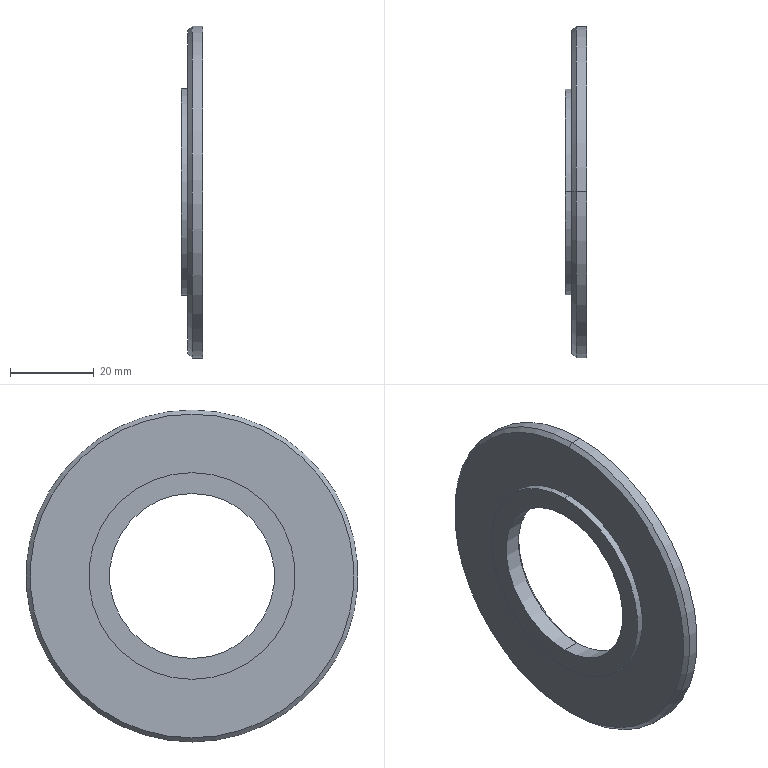Part | SolidWorks | features Chamfer 2, Revolution 1 | 1 solid | 13 faces | box 5.21 x 79.5 x 79.5 mm | volume 14367 mm3 | cylinder 6 | cone 4 | plane 3 | commonest cylinder face diameters 39.5 x2 49.5 x2 79.5 x2
STEP:
#1=CARTESIAN_POINT('',(10.713,-22.417,19.75));
#2=VERTEX_POINT('',#1);
#3=CARTESIAN_POINT('',(10.713,-22.417,-19.75));
#4=VERTEX_POINT('',#3);
#5=CARTESIAN_POINT('',(10.713,-22.417,0.));
#6=DIRECTION('',(1.,0.,0.));
#7=DIRECTION('',(0.,0.,1.));
#8=AXIS2_PLACEMENT_3D('',#5,#6,#7);
#9=CIRCLE('',#8,19.75);
#10=EDGE_CURVE('',#2,#4,#9,.T.);
#11=ORIENTED_EDGE('',*,*,#10,.F.);
#12=CARTESIAN_POINT('',(11.713,-22.417,20.75));
#13=VERTEX_POINT('',#12);
#14=CARTESIAN_POINT('',(11.713,-22.417,20.75));
#15=DIRECTION('',(0.7071,0.,0.7071));
#16=VECTOR('',#15,1000.);
#17=LINE('',#14,#16);
#18=EDGE_CURVE('',#2,#13,#17,.T.);
#19=ORIENTED_EDGE('',*,*,#18,.T.);
#20=CARTESIAN_POINT('',(11.713,-22.417,-20.75));
#21=VERTEX_POINT('',#20);
#22=CARTESIAN_POINT('',(11.713,-22.417,0.));
#23=DIRECTION('',(-1.,0.,0.));
#24=DIRECTION('',(0.,0.,1.));
#25=AXIS2_PLACEMENT_3D('',#22,#23,#24);
#26=CIRCLE('',#25,20.75);
#27=EDGE_CURVE('',#21,#13,#26,.T.);
#28=ORIENTED_EDGE('',*,*,#27,.F.);
#29=CARTESIAN_POINT('',(11.713,-22.417,-20.75));
#30=DIRECTION('',(0.7071,0.,-0.7071));
#31=VECTOR('',#30,1000.);
#32=LINE('',#29,#31);
#33=EDGE_CURVE('',#4,#21,#32,.T.);
#34=ORIENTED_EDGE('',*,*,#33,.F.);
#35=EDGE_LOOP('',(#11,#19,#28,#34));
#36=FACE_OUTER_BOUND('',#35,.T.);
#37=CARTESIAN_POINT('',(11.713,-22.417,0.));
#38=DIRECTION('',(1.,0.,0.));
#39=DIRECTION('',(0.,0.,-1.));
#40=AXIS2_PLACEMENT_3D('',#37,#38,#39);
#41=CONICAL_SURFACE('',#40,20.75,0.7854);
#42=ADVANCED_FACE('',(#36),#41,.F.);
#43=CARTESIAN_POINT('',(8.123,-22.417,38.75));
#44=VERTEX_POINT('',#43);
#45=CARTESIAN_POINT('',(8.123,-22.417,-38.75));
#46=VERTEX_POINT('',#45);
#47=CARTESIAN_POINT('',(8.123,-22.417,0.));
#48=DIRECTION('',(-1.,0.,0.));
#49=DIRECTION('',(0.,0.,-1.));
#50=AXIS2_PLACEMENT_3D('',#47,#48,#49);
#51=CIRCLE('',#50,38.75);
#52=EDGE_CURVE('',#44,#46,#51,.T.);
#53=ORIENTED_EDGE('',*,*,#52,.F.);
#54=CARTESIAN_POINT('',(9.123,-22.417,39.75));
#55=VERTEX_POINT('',#54);
#56=CARTESIAN_POINT('',(8.123,-22.417,38.75));
#57=DIRECTION('',(0.7071,0.,0.7071));
#58=VECTOR('',#57,1000.);
#59=LINE('',#56,#58);
#60=EDGE_CURVE('',#44,#55,#59,.T.);
#61=ORIENTED_EDGE('',*,*,#60,.T.);
#62=CARTESIAN_POINT('',(9.123,-22.417,-39.75));
#63=VERTEX_POINT('',#62);
#64=CARTESIAN_POINT('',(9.123,-22.417,0.));
#65=DIRECTION('',(1.,0.,0.));
#66=DIRECTION('',(0.,0.,-1.));
#67=AXIS2_PLACEMENT_3D('',#64,#65,#66);
#68=CIRCLE('',#67,39.75);
#69=EDGE_CURVE('',#63,#55,#68,.T.);
#70=ORIENTED_EDGE('',*,*,#69,.F.);
#71=CARTESIAN_POINT('',(8.123,-22.417,-38.75));
#72=DIRECTION('',(0.7071,0.,-0.7071));
#73=VECTOR('',#72,1000.);
#74=LINE('',#71,#73);
#75=EDGE_CURVE('',#46,#63,#74,.T.);
#76=ORIENTED_EDGE('',*,*,#75,.F.);
#77=EDGE_LOOP('',(#53,#61,#70,#76));
#78=FACE_OUTER_BOUND('',#77,.T.);
#79=CARTESIAN_POINT('',(8.123,-22.417,0.));
#80=DIRECTION('',(1.,0.,0.));
#81=DIRECTION('',(0.,0.,-1.));
#82=AXIS2_PLACEMENT_3D('',#79,#80,#81);
#83=CONICAL_SURFACE('',#82,38.75,0.7854);
#84=ADVANCED_FACE('',(#78),#83,.T.);
#85=CARTESIAN_POINT('',(8.123,-22.417,24.75));
#86=VERTEX_POINT('',#85);
#87=CARTESIAN_POINT('',(8.123,-22.417,-24.75));
#88=VERTEX_POINT('',#87);
#89=CARTESIAN_POINT('',(8.123,-22.417,0.));
#90=DIRECTION('',(-1.,0.,0.));
#91=DIRECTION('',(0.,0.,1.));
#92=AXIS2_PLACEMENT_3D('',#89,#90,#91);
#93=CIRCLE('',#92,24.75);
#94=EDGE_CURVE('',#86,#88,#93,.T.);
#95=ORIENTED_EDGE('',*,*,#94,.T.);
#96=CARTESIAN_POINT('',(6.503,-22.417,-24.75));
#97=VERTEX_POINT('',#96);
#98=CARTESIAN_POINT('',(4.025,-22.417,-24.75));
#99=DIRECTION('',(-1.,0.,0.));
#100=VECTOR('',#99,1000.);
#101=LINE('',#98,#100);
#102=EDGE_CURVE('',#88,#97,#101,.T.);
#103=ORIENTED_EDGE('',*,*,#102,.T.);
#104=CARTESIAN_POINT('',(6.503,-22.417,24.75));
#105=VERTEX_POINT('',#104);
#106=CARTESIAN_POINT('',(6.503,-22.417,0.));
#107=DIRECTION('',(-1.,0.,0.));
#108=DIRECTION('',(0.,0.,1.));
#109=AXIS2_PLACEMENT_3D('',#106,#107,#108);
#110=CIRCLE('',#109,24.75);
#111=EDGE_CURVE('',#105,#97,#110,.T.);
#112=ORIENTED_EDGE('',*,*,#111,.F.);
#113=CARTESIAN_POINT('',(4.025,-22.417,24.75));
#114=DIRECTION('',(-1.,0.,0.));
#115=VECTOR('',#114,1000.);
#116=LINE('',#113,#115);
#117=EDGE_CURVE('',#86,#105,#116,.T.);
#118=ORIENTED_EDGE('',*,*,#117,.F.);
#119=EDGE_LOOP('',(#95,#103,#112,#118));
#120=FACE_OUTER_BOUND('',#119,.T.);
#121=CARTESIAN_POINT('',(4.025,-22.417,0.));
#122=DIRECTION('',(-1.,0.,0.));
#123=DIRECTION('',(0.,0.,1.));
#124=AXIS2_PLACEMENT_3D('',#121,#122,#123);
#125=CYLINDRICAL_SURFACE('',#124,24.75);
#126=ADVANCED_FACE('',(#120),#125,.T.);
#127=ORIENTED_EDGE('',*,*,#10,.T.);
#128=CARTESIAN_POINT('',(6.503,-22.417,-19.75));
#129=VERTEX_POINT('',#128);
#130=CARTESIAN_POINT('',(4.025,-22.417,-19.75));
#131=DIRECTION('',(-1.,0.,0.));
#132=VECTOR('',#131,1000.);
#133=LINE('',#130,#132);
#134=EDGE_CURVE('',#4,#129,#133,.T.);
#135=ORIENTED_EDGE('',*,*,#134,.T.);
#136=CARTESIAN_POINT('',(6.503,-22.417,19.75));
#137=VERTEX_POINT('',#136);
#138=CARTESIAN_POINT('',(6.503,-22.417,0.));
#139=DIRECTION('',(-1.,0.,0.));
#140=DIRECTION('',(0.,0.,1.));
#141=AXIS2_PLACEMENT_3D('',#138,#139,#140);
#142=CIRCLE('',#141,19.75);
#143=EDGE_CURVE('',#129,#137,#142,.T.);
#144=ORIENTED_EDGE('',*,*,#143,.T.);
#145=CARTESIAN_POINT('',(4.025,-22.417,19.75));
#146=DIRECTION('',(-1.,0.,0.));
#147=VECTOR('',#146,1000.);
#148=LINE('',#145,#147);
#149=EDGE_CURVE('',#2,#137,#148,.T.);
#150=ORIENTED_EDGE('',*,*,#149,.F.);
#151=EDGE_LOOP('',(#127,#135,#144,#150));
#152=FACE_OUTER_BOUND('',#151,.T.);
#153=CARTESIAN_POINT('',(4.025,-22.417,0.));
#154=DIRECTION('',(-1.,0.,0.));
#155=DIRECTION('',(0.,0.,1.));
#156=AXIS2_PLACEMENT_3D('',#153,#154,#155);
#157=CYLINDRICAL_SURFACE('',#156,19.75);
#158=ADVANCED_FACE('',(#152),#157,.F.);
#159=CARTESIAN_POINT('',(11.713,-22.417,39.75));
#160=VERTEX_POINT('',#159);
#161=CARTESIAN_POINT('',(11.713,-22.417,-39.75));
#162=VERTEX_POINT('',#161);
#163=CARTESIAN_POINT('',(11.713,-22.417,0.));
#164=DIRECTION('',(-1.,0.,0.));
#165=DIRECTION('',(0.,0.,1.));
#166=AXIS2_PLACEMENT_3D('',#163,#164,#165);
#167=CIRCLE('',#166,39.75);
#168=EDGE_CURVE('',#160,#162,#167,.T.);
#169=ORIENTED_EDGE('',*,*,#168,.T.);
#170=CARTESIAN_POINT('',(4.025,-22.417,-39.75));
#171=DIRECTION('',(-1.,0.,0.));
#172=VECTOR('',#171,1000.);
#173=LINE('',#170,#172);
#174=EDGE_CURVE('',#162,#63,#173,.T.);
#175=ORIENTED_EDGE('',*,*,#174,.T.);
#176=ORIENTED_EDGE('',*,*,#69,.T.);
#177=CARTESIAN_POINT('',(4.025,-22.417,39.75));
#178=DIRECTION('',(-1.,0.,0.));
#179=VECTOR('',#178,1000.);
#180=LINE('',#177,#179);
#181=EDGE_CURVE('',#160,#55,#180,.T.);
#182=ORIENTED_EDGE('',*,*,#181,.F.);
#183=EDGE_LOOP('',(#169,#175,#176,#182));
#184=FACE_OUTER_BOUND('',#183,.T.);
#185=CARTESIAN_POINT('',(4.025,-22.417,0.));
#186=DIRECTION('',(-1.,0.,0.));
#187=DIRECTION('',(0.,0.,1.));
#188=AXIS2_PLACEMENT_3D('',#185,#186,#187);
#189=CYLINDRICAL_SURFACE('',#188,39.75);
#190=ADVANCED_FACE('',(#184),#189,.T.);
#191=CARTESIAN_POINT('',(8.123,-22.417,0.));
#192=DIRECTION('',(-1.,0.,0.));
#193=DIRECTION('',(0.,0.,-1.));
#194=AXIS2_PLACEMENT_3D('',#191,#192,#193);
#195=CIRCLE('',#194,38.75);
#196=EDGE_CURVE('',#46,#44,#195,.T.);
#197=ORIENTED_EDGE('',*,*,#196,.T.);
#198=ORIENTED_EDGE('',*,*,#52,.T.);
#199=EDGE_LOOP('',(#197,#198));
#200=FACE_OUTER_BOUND('',#199,.T.);
#201=ORIENTED_EDGE('',*,*,#94,.F.);
#202=CARTESIAN_POINT('',(8.123,-22.417,0.));
#203=DIRECTION('',(-1.,0.,0.));
#204=DIRECTION('',(0.,0.,1.));
#205=AXIS2_PLACEMENT_3D('',#202,#203,#204);
#206=CIRCLE('',#205,24.75);
#207=EDGE_CURVE('',#88,#86,#206,.T.);
#208=ORIENTED_EDGE('',*,*,#207,.F.);
#209=EDGE_LOOP('',(#201,#208));
#210=FACE_BOUND('',#209,.T.);
#211=CARTESIAN_POINT('',(8.123,2.333,0.));
#212=DIRECTION('',(1.,0.,0.));
#213=DIRECTION('',(0.,0.,-1.));
#214=AXIS2_PLACEMENT_3D('',#211,#212,#213);
#215=PLANE('',#214);
#216=ADVANCED_FACE('',(#200,#210),#215,.F.);
#217=ORIENTED_EDGE('',*,*,#174,.F.);
#218=CARTESIAN_POINT('',(11.713,-22.417,0.));
#219=DIRECTION('',(-1.,0.,0.));
#220=DIRECTION('',(0.,0.,1.));
#221=AXIS2_PLACEMENT_3D('',#218,#219,#220);
#222=CIRCLE('',#221,39.75);
#223=EDGE_CURVE('',#162,#160,#222,.T.);
#224=ORIENTED_EDGE('',*,*,#223,.T.);
#225=ORIENTED_EDGE('',*,*,#181,.T.);
#226=CARTESIAN_POINT('',(9.123,-22.417,0.));
#227=DIRECTION('',(1.,0.,0.));
#228=DIRECTION('',(0.,0.,-1.));
#229=AXIS2_PLACEMENT_3D('',#226,#227,#228);
#230=CIRCLE('',#229,39.75);
#231=EDGE_CURVE('',#55,#63,#230,.T.);
#232=ORIENTED_EDGE('',*,*,#231,.T.);
#233=EDGE_LOOP('',(#217,#224,#225,#232));
#234=FACE_OUTER_BOUND('',#233,.T.);
#235=CARTESIAN_POINT('',(4.025,-22.417,0.));
#236=DIRECTION('',(-1.,0.,0.));
#237=DIRECTION('',(0.,0.,1.));
#238=AXIS2_PLACEMENT_3D('',#235,#236,#237);
#239=CYLINDRICAL_SURFACE('',#238,39.75);
#240=ADVANCED_FACE('',(#234),#239,.T.);
#241=ORIENTED_EDGE('',*,*,#27,.T.);
#242=CARTESIAN_POINT('',(11.713,-22.417,0.));
#243=DIRECTION('',(-1.,0.,0.));
#244=DIRECTION('',(0.,0.,1.));
#245=AXIS2_PLACEMENT_3D('',#242,#243,#244);
#246=CIRCLE('',#245,20.75);
#247=EDGE_CURVE('',#13,#21,#246,.T.);
#248=ORIENTED_EDGE('',*,*,#247,.T.);
#249=EDGE_LOOP('',(#241,#248));
#250=FACE_BOUND('',#249,.T.);
#251=ORIENTED_EDGE('',*,*,#168,.F.);
#252=ORIENTED_EDGE('',*,*,#223,.F.);
#253=EDGE_LOOP('',(#251,#252));
#254=FACE_OUTER_BOUND('',#253,.T.);
#255=CARTESIAN_POINT('',(11.713,17.333,0.));
#256=DIRECTION('',(-1.,0.,0.));
#257=DIRECTION('',(0.,0.,1.));
#258=AXIS2_PLACEMENT_3D('',#255,#256,#257);
#259=PLANE('',#258);
#260=ADVANCED_FACE('',(#250,#254),#259,.F.);
#261=ORIENTED_EDGE('',*,*,#134,.F.);
#262=CARTESIAN_POINT('',(10.713,-22.417,0.));
#263=DIRECTION('',(1.,0.,0.));
#264=DIRECTION('',(0.,0.,1.));
#265=AXIS2_PLACEMENT_3D('',#262,#263,#264);
#266=CIRCLE('',#265,19.75);
#267=EDGE_CURVE('',#4,#2,#266,.T.);
#268=ORIENTED_EDGE('',*,*,#267,.T.);
#269=ORIENTED_EDGE('',*,*,#149,.T.);
#270=CARTESIAN_POINT('',(6.503,-22.417,0.));
#271=DIRECTION('',(-1.,0.,0.));
#272=DIRECTION('',(0.,0.,1.));
#273=AXIS2_PLACEMENT_3D('',#270,#271,#272);
#274=CIRCLE('',#273,19.75);
#275=EDGE_CURVE('',#137,#129,#274,.T.);
#276=ORIENTED_EDGE('',*,*,#275,.T.);
#277=EDGE_LOOP('',(#261,#268,#269,#276));
#278=FACE_OUTER_BOUND('',#277,.T.);
#279=CARTESIAN_POINT('',(4.025,-22.417,0.));
#280=DIRECTION('',(-1.,0.,0.));
#281=DIRECTION('',(0.,0.,1.));
#282=AXIS2_PLACEMENT_3D('',#279,#280,#281);
#283=CYLINDRICAL_SURFACE('',#282,19.75);
#284=ADVANCED_FACE('',(#278),#283,.F.);
#285=ORIENTED_EDGE('',*,*,#275,.F.);
#286=ORIENTED_EDGE('',*,*,#143,.F.);
#287=EDGE_LOOP('',(#285,#286));
#288=FACE_BOUND('',#287,.T.);
#289=ORIENTED_EDGE('',*,*,#111,.T.);
#290=CARTESIAN_POINT('',(6.503,-22.417,0.));
#291=DIRECTION('',(-1.,0.,0.));
#292=DIRECTION('',(0.,0.,1.));
#293=AXIS2_PLACEMENT_3D('',#290,#291,#292);
#294=CIRCLE('',#293,24.75);
#295=EDGE_CURVE('',#97,#105,#294,.T.);
#296=ORIENTED_EDGE('',*,*,#295,.T.);
#297=EDGE_LOOP('',(#289,#296));
#298=FACE_OUTER_BOUND('',#297,.T.);
#299=CARTESIAN_POINT('',(6.503,-2.667,0.));
#300=DIRECTION('',(1.,0.,0.));
#301=DIRECTION('',(0.,0.,-1.));
#302=AXIS2_PLACEMENT_3D('',#299,#300,#301);
#303=PLANE('',#302);
#304=ADVANCED_FACE('',(#288,#298),#303,.F.);
#305=ORIENTED_EDGE('',*,*,#102,.F.);
#306=ORIENTED_EDGE('',*,*,#207,.T.);
#307=ORIENTED_EDGE('',*,*,#117,.T.);
#308=ORIENTED_EDGE('',*,*,#295,.F.);
#309=EDGE_LOOP('',(#305,#306,#307,#308));
#310=FACE_OUTER_BOUND('',#309,.T.);
#311=CARTESIAN_POINT('',(4.025,-22.417,0.));
#312=DIRECTION('',(-1.,0.,0.));
#313=DIRECTION('',(0.,0.,1.));
#314=AXIS2_PLACEMENT_3D('',#311,#312,#313);
#315=CYLINDRICAL_SURFACE('',#314,24.75);
#316=ADVANCED_FACE('',(#310),#315,.T.);
#317=ORIENTED_EDGE('',*,*,#60,.F.);
#318=ORIENTED_EDGE('',*,*,#196,.F.);
#319=ORIENTED_EDGE('',*,*,#75,.T.);
#320=ORIENTED_EDGE('',*,*,#231,.F.);
#321=EDGE_LOOP('',(#317,#318,#319,#320));
#322=FACE_OUTER_BOUND('',#321,.T.);
#323=CARTESIAN_POINT('',(8.123,-22.417,0.));
#324=DIRECTION('',(1.,0.,0.));
#325=DIRECTION('',(0.,0.,-1.));
#326=AXIS2_PLACEMENT_3D('',#323,#324,#325);
#327=CONICAL_SURFACE('',#326,38.75,0.7854);
#328=ADVANCED_FACE('',(#322),#327,.T.);
#329=ORIENTED_EDGE('',*,*,#18,.F.);
#330=ORIENTED_EDGE('',*,*,#267,.F.);
#331=ORIENTED_EDGE('',*,*,#33,.T.);
#332=ORIENTED_EDGE('',*,*,#247,.F.);
#333=EDGE_LOOP('',(#329,#330,#331,#332));
#334=FACE_OUTER_BOUND('',#333,.T.);
#335=CARTESIAN_POINT('',(11.713,-22.417,0.));
#336=DIRECTION('',(1.,0.,0.));
#337=DIRECTION('',(0.,0.,-1.));
#338=AXIS2_PLACEMENT_3D('',#335,#336,#337);
#339=CONICAL_SURFACE('',#338,20.75,0.7854);
#340=ADVANCED_FACE('',(#334),#339,.F.);
#341=CLOSED_SHELL('',(#42,#84,#126,#158,#190,#216,#240,#260,#284,#304,#316,#328,#340));
#342=MANIFOLD_SOLID_BREP('',#341);
#343=CARTESIAN_POINT('',(0.,0.,0.));
#344=DIRECTION('',(0.,0.,1.));
#345=DIRECTION('',(1.,0.,0.));
#346=AXIS2_PLACEMENT_3D('',#343,#344,#345);
#347=(LENGTH_UNIT()NAMED_UNIT(*)SI_UNIT(.MILLI.,.METRE.));
#348=UNCERTAINTY_MEASURE_WITH_UNIT(LENGTH_MEASURE(0.00001),#347,'','');
#349=(NAMED_UNIT(*)PLANE_ANGLE_UNIT()SI_UNIT($,.RADIAN.));
#350=(NAMED_UNIT(*)SI_UNIT($,.STERADIAN.)SOLID_ANGLE_UNIT());
#351=(GEOMETRIC_REPRESENTATION_CONTEXT(3)GLOBAL_UNCERTAINTY_ASSIGNED_CONTEXT((#348))GLOBAL_UNIT_ASSIGNED_CONTEXT((#347,#349,#350))REPRESENTATION_CONTEXT('',''));
#352=ADVANCED_BREP_SHAPE_REPRESENTATION('',(#342,#346),#351);